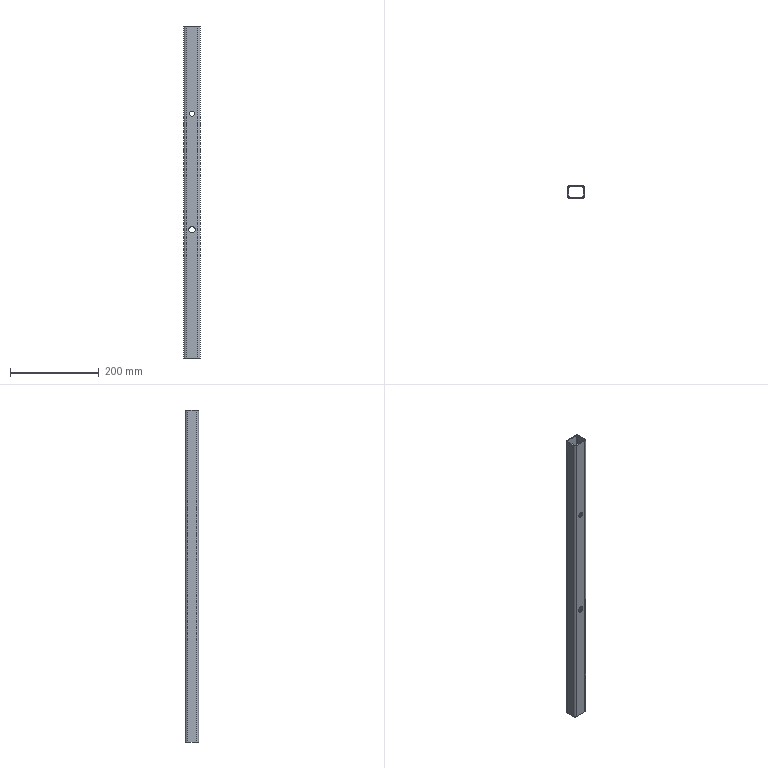Part | SolidWorks | features ICE 2, Cut 1, Extrusion 1 | 1 solid | 27 faces | box 37 x 30 x 750 mm | volume 218758 mm3 | cylinder 16 | plane 11 | commonest cylinder face diameters 5 x4 10 x4 12 x4 14 x4
STEP:
#1=CARTESIAN_POINT('',(7.,12.5,-260.));
#2=VERTEX_POINT('',#1);
#3=CARTESIAN_POINT('',(-7.,12.5,-260.));
#4=VERTEX_POINT('',#3);
#5=CARTESIAN_POINT('',(0.,12.5,-260.));
#6=DIRECTION('',(0.,1.,0.));
#7=DIRECTION('',(-1.,0.,0.));
#8=AXIS2_PLACEMENT_3D('',#5,#6,#7);
#9=CIRCLE('',#8,7.);
#10=EDGE_CURVE('',#2,#4,#9,.T.);
#11=ORIENTED_EDGE('',*,*,#10,.F.);
#12=CARTESIAN_POINT('',(7.,15.,-260.));
#13=VERTEX_POINT('',#12);
#14=CARTESIAN_POINT('',(7.,-15.,-260.));
#15=DIRECTION('',(0.,1.,0.));
#16=VECTOR('',#15,1000.);
#17=LINE('',#14,#16);
#18=EDGE_CURVE('',#2,#13,#17,.T.);
#19=ORIENTED_EDGE('',*,*,#18,.T.);
#20=CARTESIAN_POINT('',(-7.,15.,-260.));
#21=VERTEX_POINT('',#20);
#22=CARTESIAN_POINT('',(0.,15.,-260.));
#23=DIRECTION('',(0.,1.,0.));
#24=DIRECTION('',(-1.,0.,0.));
#25=AXIS2_PLACEMENT_3D('',#22,#23,#24);
#26=CIRCLE('',#25,7.);
#27=EDGE_CURVE('',#13,#21,#26,.T.);
#28=ORIENTED_EDGE('',*,*,#27,.T.);
#29=CARTESIAN_POINT('',(-7.,-15.,-260.));
#30=DIRECTION('',(0.,1.,0.));
#31=VECTOR('',#30,1000.);
#32=LINE('',#29,#31);
#33=EDGE_CURVE('',#4,#21,#32,.T.);
#34=ORIENTED_EDGE('',*,*,#33,.F.);
#35=EDGE_LOOP('',(#11,#19,#28,#34));
#36=FACE_OUTER_BOUND('',#35,.T.);
#37=CARTESIAN_POINT('',(0.,-15.,-260.));
#38=DIRECTION('',(0.,1.,0.));
#39=DIRECTION('',(-1.,0.,0.));
#40=AXIS2_PLACEMENT_3D('',#37,#38,#39);
#41=CYLINDRICAL_SURFACE('',#40,7.);
#42=ADVANCED_FACE('',(#36),#41,.F.);
#43=CARTESIAN_POINT('',(7.,-15.,-260.));
#44=VERTEX_POINT('',#43);
#45=CARTESIAN_POINT('',(-7.,-15.,-260.));
#46=VERTEX_POINT('',#45);
#47=CARTESIAN_POINT('',(0.,-15.,-260.));
#48=DIRECTION('',(0.,1.,0.));
#49=DIRECTION('',(-1.,0.,0.));
#50=AXIS2_PLACEMENT_3D('',#47,#48,#49);
#51=CIRCLE('',#50,7.);
#52=EDGE_CURVE('',#44,#46,#51,.T.);
#53=ORIENTED_EDGE('',*,*,#52,.F.);
#54=CARTESIAN_POINT('',(7.,-12.5,-260.));
#55=VERTEX_POINT('',#54);
#56=CARTESIAN_POINT('',(7.,-15.,-260.));
#57=DIRECTION('',(0.,1.,0.));
#58=VECTOR('',#57,1000.);
#59=LINE('',#56,#58);
#60=EDGE_CURVE('',#44,#55,#59,.T.);
#61=ORIENTED_EDGE('',*,*,#60,.T.);
#62=CARTESIAN_POINT('',(-7.,-12.5,-260.));
#63=VERTEX_POINT('',#62);
#64=CARTESIAN_POINT('',(0.,-12.5,-260.));
#65=DIRECTION('',(0.,-1.,0.));
#66=DIRECTION('',(1.,0.,0.));
#67=AXIS2_PLACEMENT_3D('',#64,#65,#66);
#68=CIRCLE('',#67,7.);
#69=EDGE_CURVE('',#63,#55,#68,.T.);
#70=ORIENTED_EDGE('',*,*,#69,.F.);
#71=CARTESIAN_POINT('',(-7.,-15.,-260.));
#72=DIRECTION('',(0.,1.,0.));
#73=VECTOR('',#72,1000.);
#74=LINE('',#71,#73);
#75=EDGE_CURVE('',#46,#63,#74,.T.);
#76=ORIENTED_EDGE('',*,*,#75,.F.);
#77=EDGE_LOOP('',(#53,#61,#70,#76));
#78=FACE_OUTER_BOUND('',#77,.T.);
#79=CARTESIAN_POINT('',(0.,-15.,-260.));
#80=DIRECTION('',(0.,1.,0.));
#81=DIRECTION('',(-1.,0.,0.));
#82=AXIS2_PLACEMENT_3D('',#79,#80,#81);
#83=CYLINDRICAL_SURFACE('',#82,7.);
#84=ADVANCED_FACE('',(#78),#83,.F.);
#85=CARTESIAN_POINT('',(6.,12.5,2.));
#86=VERTEX_POINT('',#85);
#87=CARTESIAN_POINT('',(-6.,12.5,2.));
#88=VERTEX_POINT('',#87);
#89=CARTESIAN_POINT('',(0.,12.5,2.));
#90=DIRECTION('',(0.,1.,0.));
#91=DIRECTION('',(-1.,0.,0.));
#92=AXIS2_PLACEMENT_3D('',#89,#90,#91);
#93=CIRCLE('',#92,6.);
#94=EDGE_CURVE('',#86,#88,#93,.T.);
#95=ORIENTED_EDGE('',*,*,#94,.F.);
#96=CARTESIAN_POINT('',(6.,15.,2.));
#97=VERTEX_POINT('',#96);
#98=CARTESIAN_POINT('',(6.,-68.,2.));
#99=DIRECTION('',(0.,1.,0.));
#100=VECTOR('',#99,1000.);
#101=LINE('',#98,#100);
#102=EDGE_CURVE('',#86,#97,#101,.T.);
#103=ORIENTED_EDGE('',*,*,#102,.T.);
#104=CARTESIAN_POINT('',(-6.,15.,2.));
#105=VERTEX_POINT('',#104);
#106=CARTESIAN_POINT('',(0.,15.,2.));
#107=DIRECTION('',(0.,1.,0.));
#108=DIRECTION('',(-1.,0.,0.));
#109=AXIS2_PLACEMENT_3D('',#106,#107,#108);
#110=CIRCLE('',#109,6.);
#111=EDGE_CURVE('',#97,#105,#110,.T.);
#112=ORIENTED_EDGE('',*,*,#111,.T.);
#113=CARTESIAN_POINT('',(-6.,-68.,2.));
#114=DIRECTION('',(0.,1.,0.));
#115=VECTOR('',#114,1000.);
#116=LINE('',#113,#115);
#117=EDGE_CURVE('',#88,#105,#116,.T.);
#118=ORIENTED_EDGE('',*,*,#117,.F.);
#119=EDGE_LOOP('',(#95,#103,#112,#118));
#120=FACE_OUTER_BOUND('',#119,.T.);
#121=CARTESIAN_POINT('',(0.,-68.,2.));
#122=DIRECTION('',(0.,1.,0.));
#123=DIRECTION('',(-1.,0.,0.));
#124=AXIS2_PLACEMENT_3D('',#121,#122,#123);
#125=CYLINDRICAL_SURFACE('',#124,6.);
#126=ADVANCED_FACE('',(#120),#125,.F.);
#127=CARTESIAN_POINT('',(-6.,-15.,2.));
#128=VERTEX_POINT('',#127);
#129=CARTESIAN_POINT('',(6.,-15.,2.));
#130=VERTEX_POINT('',#129);
#131=CARTESIAN_POINT('',(0.,-15.,2.));
#132=DIRECTION('',(0.,-1.,0.));
#133=DIRECTION('',(1.,0.,0.));
#134=AXIS2_PLACEMENT_3D('',#131,#132,#133);
#135=CIRCLE('',#134,6.);
#136=EDGE_CURVE('',#128,#130,#135,.T.);
#137=ORIENTED_EDGE('',*,*,#136,.T.);
#138=CARTESIAN_POINT('',(6.,-12.5,2.));
#139=VERTEX_POINT('',#138);
#140=CARTESIAN_POINT('',(6.,-68.,2.));
#141=DIRECTION('',(0.,1.,0.));
#142=VECTOR('',#141,1000.);
#143=LINE('',#140,#142);
#144=EDGE_CURVE('',#130,#139,#143,.T.);
#145=ORIENTED_EDGE('',*,*,#144,.T.);
#146=CARTESIAN_POINT('',(-6.,-12.5,2.));
#147=VERTEX_POINT('',#146);
#148=CARTESIAN_POINT('',(0.,-12.5,2.));
#149=DIRECTION('',(0.,-1.,0.));
#150=DIRECTION('',(1.,0.,0.));
#151=AXIS2_PLACEMENT_3D('',#148,#149,#150);
#152=CIRCLE('',#151,6.);
#153=EDGE_CURVE('',#147,#139,#152,.T.);
#154=ORIENTED_EDGE('',*,*,#153,.F.);
#155=CARTESIAN_POINT('',(-6.,-68.,2.));
#156=DIRECTION('',(0.,1.,0.));
#157=VECTOR('',#156,1000.);
#158=LINE('',#155,#157);
#159=EDGE_CURVE('',#128,#147,#158,.T.);
#160=ORIENTED_EDGE('',*,*,#159,.F.);
#161=EDGE_LOOP('',(#137,#145,#154,#160));
#162=FACE_OUTER_BOUND('',#161,.T.);
#163=CARTESIAN_POINT('',(0.,-68.,2.));
#164=DIRECTION('',(0.,1.,0.));
#165=DIRECTION('',(-1.,0.,0.));
#166=AXIS2_PLACEMENT_3D('',#163,#164,#165);
#167=CYLINDRICAL_SURFACE('',#166,6.);
#168=ADVANCED_FACE('',(#162),#167,.F.);
#169=CARTESIAN_POINT('',(-13.5,-15.,-550.));
#170=VERTEX_POINT('',#169);
#171=CARTESIAN_POINT('',(-13.5,-15.,200.));
#172=VERTEX_POINT('',#171);
#173=CARTESIAN_POINT('',(-13.5,-15.,-300.));
#174=DIRECTION('',(0.,0.,1.));
#175=VECTOR('',#174,1000.);
#176=LINE('',#173,#175);
#177=EDGE_CURVE('',#170,#172,#176,.T.);
#178=ORIENTED_EDGE('',*,*,#177,.T.);
#179=CARTESIAN_POINT('',(-18.5,-10.,200.));
#180=VERTEX_POINT('',#179);
#181=CARTESIAN_POINT('',(-13.5,-10.,200.));
#182=DIRECTION('',(0.,0.,1.));
#183=DIRECTION('',(1.,0.,0.));
#184=AXIS2_PLACEMENT_3D('',#181,#182,#183);
#185=CIRCLE('',#184,5.);
#186=EDGE_CURVE('',#180,#172,#185,.T.);
#187=ORIENTED_EDGE('',*,*,#186,.F.);
#188=CARTESIAN_POINT('',(-18.5,-10.,-550.));
#189=VERTEX_POINT('',#188);
#190=CARTESIAN_POINT('',(-18.5,-10.,-300.));
#191=DIRECTION('',(0.,0.,1.));
#192=VECTOR('',#191,1000.);
#193=LINE('',#190,#192);
#194=EDGE_CURVE('',#189,#180,#193,.T.);
#195=ORIENTED_EDGE('',*,*,#194,.F.);
#196=CARTESIAN_POINT('',(-13.5,-10.,-550.));
#197=DIRECTION('',(0.,0.,-1.));
#198=DIRECTION('',(-1.,0.,0.));
#199=AXIS2_PLACEMENT_3D('',#196,#197,#198);
#200=CIRCLE('',#199,5.);
#201=EDGE_CURVE('',#170,#189,#200,.T.);
#202=ORIENTED_EDGE('',*,*,#201,.F.);
#203=EDGE_LOOP('',(#178,#187,#195,#202));
#204=FACE_OUTER_BOUND('',#203,.T.);
#205=CARTESIAN_POINT('',(-13.5,-10.,-300.));
#206=DIRECTION('',(0.,0.,1.));
#207=DIRECTION('',(1.,0.,0.));
#208=AXIS2_PLACEMENT_3D('',#205,#206,#207);
#209=CYLINDRICAL_SURFACE('',#208,5.);
#210=ADVANCED_FACE('',(#204),#209,.T.);
#211=ORIENTED_EDGE('',*,*,#194,.T.);
#212=CARTESIAN_POINT('',(-18.5,10.,200.));
#213=VERTEX_POINT('',#212);
#214=CARTESIAN_POINT('',(-18.5,10.,200.));
#215=DIRECTION('',(0.,-1.,0.));
#216=VECTOR('',#215,1000.);
#217=LINE('',#214,#216);
#218=EDGE_CURVE('',#213,#180,#217,.T.);
#219=ORIENTED_EDGE('',*,*,#218,.F.);
#220=CARTESIAN_POINT('',(-18.5,10.,-550.));
#221=VERTEX_POINT('',#220);
#222=CARTESIAN_POINT('',(-18.5,10.,-300.));
#223=DIRECTION('',(0.,0.,1.));
#224=VECTOR('',#223,1000.);
#225=LINE('',#222,#224);
#226=EDGE_CURVE('',#221,#213,#225,.T.);
#227=ORIENTED_EDGE('',*,*,#226,.F.);
#228=CARTESIAN_POINT('',(-18.5,-10.,-550.));
#229=DIRECTION('',(0.,1.,0.));
#230=VECTOR('',#229,1000.);
#231=LINE('',#228,#230);
#232=EDGE_CURVE('',#189,#221,#231,.T.);
#233=ORIENTED_EDGE('',*,*,#232,.F.);
#234=EDGE_LOOP('',(#211,#219,#227,#233));
#235=FACE_OUTER_BOUND('',#234,.T.);
#236=CARTESIAN_POINT('',(-18.5,10.,-300.));
#237=DIRECTION('',(-1.,0.,0.));
#238=DIRECTION('',(0.,0.,1.));
#239=AXIS2_PLACEMENT_3D('',#236,#237,#238);
#240=PLANE('',#239);
#241=ADVANCED_FACE('',(#235),#240,.T.);
#242=ORIENTED_EDGE('',*,*,#226,.T.);
#243=CARTESIAN_POINT('',(-13.5,15.,200.));
#244=VERTEX_POINT('',#243);
#245=CARTESIAN_POINT('',(-13.5,10.,200.));
#246=DIRECTION('',(0.,0.,1.));
#247=DIRECTION('',(1.,0.,0.));
#248=AXIS2_PLACEMENT_3D('',#245,#246,#247);
#249=CIRCLE('',#248,5.);
#250=EDGE_CURVE('',#244,#213,#249,.T.);
#251=ORIENTED_EDGE('',*,*,#250,.F.);
#252=CARTESIAN_POINT('',(-13.5,15.,-550.));
#253=VERTEX_POINT('',#252);
#254=CARTESIAN_POINT('',(-13.5,15.,-300.));
#255=DIRECTION('',(0.,0.,1.));
#256=VECTOR('',#255,1000.);
#257=LINE('',#254,#256);
#258=EDGE_CURVE('',#253,#244,#257,.T.);
#259=ORIENTED_EDGE('',*,*,#258,.F.);
#260=CARTESIAN_POINT('',(-13.5,10.,-550.));
#261=DIRECTION('',(0.,0.,-1.));
#262=DIRECTION('',(-1.,0.,0.));
#263=AXIS2_PLACEMENT_3D('',#260,#261,#262);
#264=CIRCLE('',#263,5.);
#265=EDGE_CURVE('',#221,#253,#264,.T.);
#266=ORIENTED_EDGE('',*,*,#265,.F.);
#267=EDGE_LOOP('',(#242,#251,#259,#266));
#268=FACE_OUTER_BOUND('',#267,.T.);
#269=CARTESIAN_POINT('',(-13.5,10.,-300.));
#270=DIRECTION('',(0.,0.,1.));
#271=DIRECTION('',(1.,0.,0.));
#272=AXIS2_PLACEMENT_3D('',#269,#270,#271);
#273=CYLINDRICAL_SURFACE('',#272,5.);
#274=ADVANCED_FACE('',(#268),#273,.T.);
#275=CARTESIAN_POINT('',(0.,15.,-260.));
#276=DIRECTION('',(0.,1.,0.));
#277=DIRECTION('',(-1.,0.,0.));
#278=AXIS2_PLACEMENT_3D('',#275,#276,#277);
#279=CIRCLE('',#278,7.);
#280=EDGE_CURVE('',#21,#13,#279,.T.);
#281=ORIENTED_EDGE('',*,*,#280,.F.);
#282=ORIENTED_EDGE('',*,*,#27,.F.);
#283=EDGE_LOOP('',(#281,#282));
#284=FACE_BOUND('',#283,.T.);
#285=CARTESIAN_POINT('',(0.,15.,2.));
#286=DIRECTION('',(0.,1.,0.));
#287=DIRECTION('',(-1.,0.,0.));
#288=AXIS2_PLACEMENT_3D('',#285,#286,#287);
#289=CIRCLE('',#288,6.);
#290=EDGE_CURVE('',#105,#97,#289,.T.);
#291=ORIENTED_EDGE('',*,*,#290,.F.);
#292=ORIENTED_EDGE('',*,*,#111,.F.);
#293=EDGE_LOOP('',(#291,#292));
#294=FACE_BOUND('',#293,.T.);
#295=ORIENTED_EDGE('',*,*,#258,.T.);
#296=CARTESIAN_POINT('',(13.5,15.,200.));
#297=VERTEX_POINT('',#296);
#298=CARTESIAN_POINT('',(-13.5,15.,200.));
#299=DIRECTION('',(-1.,0.,0.));
#300=VECTOR('',#299,1000.);
#301=LINE('',#298,#300);
#302=EDGE_CURVE('',#297,#244,#301,.T.);
#303=ORIENTED_EDGE('',*,*,#302,.F.);
#304=CARTESIAN_POINT('',(13.5,15.,-550.));
#305=VERTEX_POINT('',#304);
#306=CARTESIAN_POINT('',(13.5,15.,-300.));
#307=DIRECTION('',(0.,0.,1.));
#308=VECTOR('',#307,1000.);
#309=LINE('',#306,#308);
#310=EDGE_CURVE('',#305,#297,#309,.T.);
#311=ORIENTED_EDGE('',*,*,#310,.F.);
#312=CARTESIAN_POINT('',(-13.5,15.,-550.));
#313=DIRECTION('',(1.,0.,0.));
#314=VECTOR('',#313,1000.);
#315=LINE('',#312,#314);
#316=EDGE_CURVE('',#253,#305,#315,.T.);
#317=ORIENTED_EDGE('',*,*,#316,.F.);
#318=EDGE_LOOP('',(#295,#303,#311,#317));
#319=FACE_OUTER_BOUND('',#318,.T.);
#320=CARTESIAN_POINT('',(-13.5,15.,-300.));
#321=DIRECTION('',(0.,1.,0.));
#322=DIRECTION('',(-1.,0.,0.));
#323=AXIS2_PLACEMENT_3D('',#320,#321,#322);
#324=PLANE('',#323);
#325=ADVANCED_FACE('',(#284,#294,#319),#324,.T.);
#326=ORIENTED_EDGE('',*,*,#310,.T.);
#327=CARTESIAN_POINT('',(18.5,10.,200.));
#328=VERTEX_POINT('',#327);
#329=CARTESIAN_POINT('',(13.5,10.,200.));
#330=DIRECTION('',(0.,0.,1.));
#331=DIRECTION('',(-1.,0.,0.));
#332=AXIS2_PLACEMENT_3D('',#329,#330,#331);
#333=CIRCLE('',#332,5.);
#334=EDGE_CURVE('',#328,#297,#333,.T.);
#335=ORIENTED_EDGE('',*,*,#334,.F.);
#336=CARTESIAN_POINT('',(18.5,10.,-550.));
#337=VERTEX_POINT('',#336);
#338=CARTESIAN_POINT('',(18.5,10.,-300.));
#339=DIRECTION('',(0.,0.,1.));
#340=VECTOR('',#339,1000.);
#341=LINE('',#338,#340);
#342=EDGE_CURVE('',#337,#328,#341,.T.);
#343=ORIENTED_EDGE('',*,*,#342,.F.);
#344=CARTESIAN_POINT('',(13.5,10.,-550.));
#345=DIRECTION('',(0.,0.,-1.));
#346=DIRECTION('',(-1.,0.,0.));
#347=AXIS2_PLACEMENT_3D('',#344,#345,#346);
#348=CIRCLE('',#347,5.);
#349=EDGE_CURVE('',#305,#337,#348,.T.);
#350=ORIENTED_EDGE('',*,*,#349,.F.);
#351=EDGE_LOOP('',(#326,#335,#343,#350));
#352=FACE_OUTER_BOUND('',#351,.T.);
#353=CARTESIAN_POINT('',(13.5,10.,-300.));
#354=DIRECTION('',(0.,0.,1.));
#355=DIRECTION('',(1.,0.,0.));
#356=AXIS2_PLACEMENT_3D('',#353,#354,#355);
#357=CYLINDRICAL_SURFACE('',#356,5.);
#358=ADVANCED_FACE('',(#352),#357,.T.);
#359=ORIENTED_EDGE('',*,*,#342,.T.);
#360=CARTESIAN_POINT('',(18.5,-10.,200.));
#361=VERTEX_POINT('',#360);
#362=CARTESIAN_POINT('',(18.5,10.,200.));
#363=DIRECTION('',(0.,1.,0.));
#364=VECTOR('',#363,1000.);
#365=LINE('',#362,#364);
#366=EDGE_CURVE('',#361,#328,#365,.T.);
#367=ORIENTED_EDGE('',*,*,#366,.F.);
#368=CARTESIAN_POINT('',(18.5,-10.,-550.));
#369=VERTEX_POINT('',#368);
#370=CARTESIAN_POINT('',(18.5,-10.,-300.));
#371=DIRECTION('',(0.,0.,1.));
#372=VECTOR('',#371,1000.);
#373=LINE('',#370,#372);
#374=EDGE_CURVE('',#369,#361,#373,.T.);
#375=ORIENTED_EDGE('',*,*,#374,.F.);
#376=CARTESIAN_POINT('',(18.5,10.,-550.));
#377=DIRECTION('',(0.,-1.,0.));
#378=VECTOR('',#377,1000.);
#379=LINE('',#376,#378);
#380=EDGE_CURVE('',#337,#369,#379,.T.);
#381=ORIENTED_EDGE('',*,*,#380,.F.);
#382=EDGE_LOOP('',(#359,#367,#375,#381));
#383=FACE_OUTER_BOUND('',#382,.T.);
#384=CARTESIAN_POINT('',(18.5,10.,-300.));
#385=DIRECTION('',(1.,0.,0.));
#386=DIRECTION('',(0.,0.,-1.));
#387=AXIS2_PLACEMENT_3D('',#384,#385,#386);
#388=PLANE('',#387);
#389=ADVANCED_FACE('',(#383),#388,.T.);
#390=ORIENTED_EDGE('',*,*,#374,.T.);
#391=CARTESIAN_POINT('',(13.5,-15.,200.));
#392=VERTEX_POINT('',#391);
#393=CARTESIAN_POINT('',(13.5,-10.,200.));
#394=DIRECTION('',(0.,0.,1.));
#395=DIRECTION('',(1.,0.,0.));
#396=AXIS2_PLACEMENT_3D('',#393,#394,#395);
#397=CIRCLE('',#396,5.);
#398=EDGE_CURVE('',#392,#361,#397,.T.);
#399=ORIENTED_EDGE('',*,*,#398,.F.);
#400=CARTESIAN_POINT('',(13.5,-15.,-550.));
#401=VERTEX_POINT('',#400);
#402=CARTESIAN_POINT('',(13.5,-15.,-300.));
#403=DIRECTION('',(0.,0.,1.));
#404=VECTOR('',#403,1000.);
#405=LINE('',#402,#404);
#406=EDGE_CURVE('',#401,#392,#405,.T.);
#407=ORIENTED_EDGE('',*,*,#406,.F.);
#408=CARTESIAN_POINT('',(13.5,-10.,-550.));
#409=DIRECTION('',(0.,0.,-1.));
#410=DIRECTION('',(-1.,0.,0.));
#411=AXIS2_PLACEMENT_3D('',#408,#409,#410);
#412=CIRCLE('',#411,5.);
#413=EDGE_CURVE('',#369,#401,#412,.T.);
#414=ORIENTED_EDGE('',*,*,#413,.F.);
#415=EDGE_LOOP('',(#390,#399,#407,#414));
#416=FACE_OUTER_BOUND('',#415,.T.);
#417=CARTESIAN_POINT('',(13.5,-10.,-300.));
#418=DIRECTION('',(0.,0.,1.));
#419=DIRECTION('',(1.,0.,0.));
#420=AXIS2_PLACEMENT_3D('',#417,#418,#419);
#421=CYLINDRICAL_SURFACE('',#420,5.);
#422=ADVANCED_FACE('',(#416),#421,.T.);
#423=CARTESIAN_POINT('',(0.,-15.,-260.));
#424=DIRECTION('',(0.,1.,0.));
#425=DIRECTION('',(-1.,0.,0.));
#426=AXIS2_PLACEMENT_3D('',#423,#424,#425);
#427=CIRCLE('',#426,7.);
#428=EDGE_CURVE('',#46,#44,#427,.T.);
#429=ORIENTED_EDGE('',*,*,#428,.T.);
#430=ORIENTED_EDGE('',*,*,#52,.T.);
#431=EDGE_LOOP('',(#429,#430));
#432=FACE_BOUND('',#431,.T.);
#433=ORIENTED_EDGE('',*,*,#136,.F.);
#434=CARTESIAN_POINT('',(0.,-15.,2.));
#435=DIRECTION('',(0.,-1.,0.));
#436=DIRECTION('',(1.,0.,0.));
#437=AXIS2_PLACEMENT_3D('',#434,#435,#436);
#438=CIRCLE('',#437,6.);
#439=EDGE_CURVE('',#130,#128,#438,.T.);
#440=ORIENTED_EDGE('',*,*,#439,.F.);
#441=EDGE_LOOP('',(#433,#440));
#442=FACE_BOUND('',#441,.T.);
#443=ORIENTED_EDGE('',*,*,#406,.T.);
#444=CARTESIAN_POINT('',(-13.5,-15.,200.));
#445=DIRECTION('',(1.,0.,0.));
#446=VECTOR('',#445,1000.);
#447=LINE('',#444,#446);
#448=EDGE_CURVE('',#172,#392,#447,.T.);
#449=ORIENTED_EDGE('',*,*,#448,.F.);
#450=ORIENTED_EDGE('',*,*,#177,.F.);
#451=CARTESIAN_POINT('',(13.5,-15.,-550.));
#452=DIRECTION('',(-1.,0.,0.));
#453=VECTOR('',#452,1000.);
#454=LINE('',#451,#453);
#455=EDGE_CURVE('',#401,#170,#454,.T.);
#456=ORIENTED_EDGE('',*,*,#455,.F.);
#457=EDGE_LOOP('',(#443,#449,#450,#456));
#458=FACE_OUTER_BOUND('',#457,.T.);
#459=CARTESIAN_POINT('',(-13.5,-15.,-300.));
#460=DIRECTION('',(0.,-1.,0.));
#461=DIRECTION('',(1.,0.,0.));
#462=AXIS2_PLACEMENT_3D('',#459,#460,#461);
#463=PLANE('',#462);
#464=ADVANCED_FACE('',(#432,#442,#458),#463,.T.);
#465=CARTESIAN_POINT('',(13.5,-12.5,-300.));
#466=VERTEX_POINT('',#465);
#467=CARTESIAN_POINT('',(16.,-10.,-300.));
#468=VERTEX_POINT('',#467);
#469=CARTESIAN_POINT('',(13.5,-10.,-300.));
#470=DIRECTION('',(0.,0.,1.));
#471=DIRECTION('',(-1.,0.,0.));
#472=AXIS2_PLACEMENT_3D('',#469,#470,#471);
#473=CIRCLE('',#472,2.5);
#474=EDGE_CURVE('',#466,#468,#473,.T.);
#475=ORIENTED_EDGE('',*,*,#474,.T.);
#476=CARTESIAN_POINT('',(16.,-12.5,-300.));
#477=VERTEX_POINT('',#476);
#478=CARTESIAN_POINT('',(16.,-12.5,-300.));
#479=DIRECTION('',(0.,-1.,0.));
#480=VECTOR('',#479,1000.);
#481=LINE('',#478,#480);
#482=EDGE_CURVE('',#468,#477,#481,.T.);
#483=ORIENTED_EDGE('',*,*,#482,.T.);
#484=CARTESIAN_POINT('',(16.,-12.5,-300.));
#485=DIRECTION('',(-1.,0.,0.));
#486=VECTOR('',#485,1000.);
#487=LINE('',#484,#486);
#488=EDGE_CURVE('',#477,#466,#487,.T.);
#489=ORIENTED_EDGE('',*,*,#488,.T.);
#490=EDGE_LOOP('',(#475,#483,#489));
#491=FACE_OUTER_BOUND('',#490,.T.);
#492=CARTESIAN_POINT('',(-13.5,-10.,-300.));
#493=DIRECTION('',(0.,0.,1.));
#494=DIRECTION('',(1.,0.,0.));
#495=AXIS2_PLACEMENT_3D('',#492,#493,#494);
#496=PLANE('',#495);
#497=ADVANCED_FACE('',(#491),#496,.F.);
#498=CARTESIAN_POINT('',(-16.,-10.,-550.));
#499=VERTEX_POINT('',#498);
#500=CARTESIAN_POINT('',(-16.,-10.,200.));
#501=VERTEX_POINT('',#500);
#502=CARTESIAN_POINT('',(-16.,-10.,-300.));
#503=DIRECTION('',(0.,0.,1.));
#504=VECTOR('',#503,1000.);
#505=LINE('',#502,#504);
#506=EDGE_CURVE('',#499,#501,#505,.T.);
#507=ORIENTED_EDGE('',*,*,#506,.T.);
#508=CARTESIAN_POINT('',(-13.5,-12.5,200.));
#509=VERTEX_POINT('',#508);
#510=CARTESIAN_POINT('',(-13.5,-10.,200.));
#511=DIRECTION('',(0.,0.,1.));
#512=DIRECTION('',(-1.,0.,0.));
#513=AXIS2_PLACEMENT_3D('',#510,#511,#512);
#514=CIRCLE('',#513,2.5);
#515=EDGE_CURVE('',#501,#509,#514,.T.);
#516=ORIENTED_EDGE('',*,*,#515,.T.);
#517=CARTESIAN_POINT('',(-13.5,-12.5,-550.));
#518=VERTEX_POINT('',#517);
#519=CARTESIAN_POINT('',(-13.5,-12.5,-300.));
#520=DIRECTION('',(0.,0.,1.));
#521=VECTOR('',#520,1000.);
#522=LINE('',#519,#521);
#523=EDGE_CURVE('',#518,#509,#522,.T.);
#524=ORIENTED_EDGE('',*,*,#523,.F.);
#525=CARTESIAN_POINT('',(-13.5,-10.,-550.));
#526=DIRECTION('',(0.,0.,-1.));
#527=DIRECTION('',(-1.,0.,0.));
#528=AXIS2_PLACEMENT_3D('',#525,#526,#527);
#529=CIRCLE('',#528,2.5);
#530=EDGE_CURVE('',#518,#499,#529,.T.);
#531=ORIENTED_EDGE('',*,*,#530,.T.);
#532=EDGE_LOOP('',(#507,#516,#524,#531));
#533=FACE_OUTER_BOUND('',#532,.T.);
#534=CARTESIAN_POINT('',(-13.5,-10.,-300.));
#535=DIRECTION('',(0.,0.,1.));
#536=DIRECTION('',(1.,0.,0.));
#537=AXIS2_PLACEMENT_3D('',#534,#535,#536);
#538=CYLINDRICAL_SURFACE('',#537,2.5);
#539=ADVANCED_FACE('',(#533),#538,.F.);
#540=CARTESIAN_POINT('',(-16.,10.,-550.));
#541=VERTEX_POINT('',#540);
#542=CARTESIAN_POINT('',(-16.,10.,200.));
#543=VERTEX_POINT('',#542);
#544=CARTESIAN_POINT('',(-16.,10.,-300.));
#545=DIRECTION('',(0.,0.,1.));
#546=VECTOR('',#545,1000.);
#547=LINE('',#544,#546);
#548=EDGE_CURVE('',#541,#543,#547,.T.);
#549=ORIENTED_EDGE('',*,*,#548,.T.);
#550=CARTESIAN_POINT('',(-16.,10.,200.));
#551=DIRECTION('',(0.,-1.,0.));
#552=VECTOR('',#551,1000.);
#553=LINE('',#550,#552);
#554=EDGE_CURVE('',#543,#501,#553,.T.);
#555=ORIENTED_EDGE('',*,*,#554,.T.);
#556=ORIENTED_EDGE('',*,*,#506,.F.);
#557=CARTESIAN_POINT('',(-16.,-10.,-550.));
#558=DIRECTION('',(0.,1.,0.));
#559=VECTOR('',#558,1000.);
#560=LINE('',#557,#559);
#561=EDGE_CURVE('',#499,#541,#560,.T.);
#562=ORIENTED_EDGE('',*,*,#561,.T.);
#563=EDGE_LOOP('',(#549,#555,#556,#562));
#564=FACE_OUTER_BOUND('',#563,.T.);
#565=CARTESIAN_POINT('',(-16.,10.,-300.));
#566=DIRECTION('',(-1.,0.,0.));
#567=DIRECTION('',(0.,0.,1.));
#568=AXIS2_PLACEMENT_3D('',#565,#566,#567);
#569=PLANE('',#568);
#570=ADVANCED_FACE('',(#564),#569,.F.);
#571=CARTESIAN_POINT('',(-13.5,12.5,-550.));
#572=VERTEX_POINT('',#571);
#573=CARTESIAN_POINT('',(-13.5,12.5,200.));
#574=VERTEX_POINT('',#573);
#575=CARTESIAN_POINT('',(-13.5,12.5,-300.));
#576=DIRECTION('',(0.,0.,1.));
#577=VECTOR('',#576,1000.);
#578=LINE('',#575,#577);
#579=EDGE_CURVE('',#572,#574,#578,.T.);
#580=ORIENTED_EDGE('',*,*,#579,.T.);
#581=CARTESIAN_POINT('',(-13.5,10.,200.));
#582=DIRECTION('',(0.,0.,1.));
#583=DIRECTION('',(1.,0.,0.));
#584=AXIS2_PLACEMENT_3D('',#581,#582,#583);
#585=CIRCLE('',#584,2.5);
#586=EDGE_CURVE('',#574,#543,#585,.T.);
#587=ORIENTED_EDGE('',*,*,#586,.T.);
#588=ORIENTED_EDGE('',*,*,#548,.F.);
#589=CARTESIAN_POINT('',(-13.5,10.,-550.));
#590=DIRECTION('',(0.,0.,-1.));
#591=DIRECTION('',(-1.,0.,0.));
#592=AXIS2_PLACEMENT_3D('',#589,#590,#591);
#593=CIRCLE('',#592,2.5);
#594=EDGE_CURVE('',#541,#572,#593,.T.);
#595=ORIENTED_EDGE('',*,*,#594,.T.);
#596=EDGE_LOOP('',(#580,#587,#588,#595));
#597=FACE_OUTER_BOUND('',#596,.T.);
#598=CARTESIAN_POINT('',(-13.5,10.,-300.));
#599=DIRECTION('',(0.,0.,1.));
#600=DIRECTION('',(1.,0.,0.));
#601=AXIS2_PLACEMENT_3D('',#598,#599,#600);
#602=CYLINDRICAL_SURFACE('',#601,2.5);
#603=ADVANCED_FACE('',(#597),#602,.F.);
#604=CARTESIAN_POINT('',(0.,12.5,-260.));
#605=DIRECTION('',(0.,1.,0.));
#606=DIRECTION('',(-1.,0.,0.));
#607=AXIS2_PLACEMENT_3D('',#604,#605,#606);
#608=CIRCLE('',#607,7.);
#609=EDGE_CURVE('',#4,#2,#608,.T.);
#610=ORIENTED_EDGE('',*,*,#609,.T.);
#611=ORIENTED_EDGE('',*,*,#10,.T.);
#612=EDGE_LOOP('',(#610,#611));
#613=FACE_BOUND('',#612,.T.);
#614=CARTESIAN_POINT('',(0.,12.5,2.));
#615=DIRECTION('',(0.,1.,0.));
#616=DIRECTION('',(-1.,0.,0.));
#617=AXIS2_PLACEMENT_3D('',#614,#615,#616);
#618=CIRCLE('',#617,6.);
#619=EDGE_CURVE('',#88,#86,#618,.T.);
#620=ORIENTED_EDGE('',*,*,#619,.T.);
#621=ORIENTED_EDGE('',*,*,#94,.T.);
#622=EDGE_LOOP('',(#620,#621));
#623=FACE_BOUND('',#622,.T.);
#624=CARTESIAN_POINT('',(13.5,12.5,-550.));
#625=VERTEX_POINT('',#624);
#626=CARTESIAN_POINT('',(13.5,12.5,200.));
#627=VERTEX_POINT('',#626);
#628=CARTESIAN_POINT('',(13.5,12.5,-300.));
#629=DIRECTION('',(0.,0.,1.));
#630=VECTOR('',#629,1000.);
#631=LINE('',#628,#630);
#632=EDGE_CURVE('',#625,#627,#631,.T.);
#633=ORIENTED_EDGE('',*,*,#632,.T.);
#634=CARTESIAN_POINT('',(-13.5,12.5,200.));
#635=DIRECTION('',(-1.,0.,0.));
#636=VECTOR('',#635,1000.);
#637=LINE('',#634,#636);
#638=EDGE_CURVE('',#627,#574,#637,.T.);
#639=ORIENTED_EDGE('',*,*,#638,.T.);
#640=ORIENTED_EDGE('',*,*,#579,.F.);
#641=CARTESIAN_POINT('',(13.5,12.5,-550.));
#642=DIRECTION('',(1.,0.,0.));
#643=VECTOR('',#642,1000.);
#644=LINE('',#641,#643);
#645=EDGE_CURVE('',#572,#625,#644,.T.);
#646=ORIENTED_EDGE('',*,*,#645,.T.);
#647=EDGE_LOOP('',(#633,#639,#640,#646));
#648=FACE_OUTER_BOUND('',#647,.T.);
#649=CARTESIAN_POINT('',(-13.5,12.5,-300.));
#650=DIRECTION('',(0.,1.,0.));
#651=DIRECTION('',(-1.,0.,0.));
#652=AXIS2_PLACEMENT_3D('',#649,#650,#651);
#653=PLANE('',#652);
#654=ADVANCED_FACE('',(#613,#623,#648),#653,.F.);
#655=CARTESIAN_POINT('',(16.,10.,-550.));
#656=VERTEX_POINT('',#655);
#657=CARTESIAN_POINT('',(16.,10.,200.));
#658=VERTEX_POINT('',#657);
#659=CARTESIAN_POINT('',(16.,10.,-300.));
#660=DIRECTION('',(0.,0.,1.));
#661=VECTOR('',#660,1000.);
#662=LINE('',#659,#661);
#663=EDGE_CURVE('',#656,#658,#662,.T.);
#664=ORIENTED_EDGE('',*,*,#663,.T.);
#665=CARTESIAN_POINT('',(13.5,10.,200.));
#666=DIRECTION('',(0.,0.,1.));
#667=DIRECTION('',(-1.,0.,0.));
#668=AXIS2_PLACEMENT_3D('',#665,#666,#667);
#669=CIRCLE('',#668,2.5);
#670=EDGE_CURVE('',#658,#627,#669,.T.);
#671=ORIENTED_EDGE('',*,*,#670,.T.);
#672=ORIENTED_EDGE('',*,*,#632,.F.);
#673=CARTESIAN_POINT('',(13.5,10.,-550.));
#674=DIRECTION('',(0.,0.,-1.));
#675=DIRECTION('',(1.,0.,0.));
#676=AXIS2_PLACEMENT_3D('',#673,#674,#675);
#677=CIRCLE('',#676,2.5);
#678=EDGE_CURVE('',#625,#656,#677,.T.);
#679=ORIENTED_EDGE('',*,*,#678,.T.);
#680=EDGE_LOOP('',(#664,#671,#672,#679));
#681=FACE_OUTER_BOUND('',#680,.T.);
#682=CARTESIAN_POINT('',(13.5,10.,-300.));
#683=DIRECTION('',(0.,0.,1.));
#684=DIRECTION('',(1.,0.,0.));
#685=AXIS2_PLACEMENT_3D('',#682,#683,#684);
#686=CYLINDRICAL_SURFACE('',#685,2.5);
#687=ADVANCED_FACE('',(#681),#686,.F.);
#688=CARTESIAN_POINT('',(16.,-10.,200.));
#689=VERTEX_POINT('',#688);
#690=CARTESIAN_POINT('',(16.,-10.,-300.));
#691=DIRECTION('',(0.,0.,1.));
#692=VECTOR('',#691,1000.);
#693=LINE('',#690,#692);
#694=EDGE_CURVE('',#468,#689,#693,.T.);
#695=ORIENTED_EDGE('',*,*,#694,.T.);
#696=CARTESIAN_POINT('',(16.,10.,200.));
#697=DIRECTION('',(0.,1.,0.));
#698=VECTOR('',#697,1000.);
#699=LINE('',#696,#698);
#700=EDGE_CURVE('',#689,#658,#699,.T.);
#701=ORIENTED_EDGE('',*,*,#700,.T.);
#702=ORIENTED_EDGE('',*,*,#663,.F.);
#703=CARTESIAN_POINT('',(16.,-12.5,-550.));
#704=VERTEX_POINT('',#703);
#705=CARTESIAN_POINT('',(16.,-12.5,-550.));
#706=DIRECTION('',(0.,-1.,0.));
#707=VECTOR('',#706,1000.);
#708=LINE('',#705,#707);
#709=EDGE_CURVE('',#656,#704,#708,.T.);
#710=ORIENTED_EDGE('',*,*,#709,.T.);
#711=CARTESIAN_POINT('',(16.,-12.5,-550.));
#712=DIRECTION('',(0.,0.,1.));
#713=VECTOR('',#712,1000.);
#714=LINE('',#711,#713);
#715=EDGE_CURVE('',#704,#477,#714,.T.);
#716=ORIENTED_EDGE('',*,*,#715,.T.);
#717=ORIENTED_EDGE('',*,*,#482,.F.);
#718=EDGE_LOOP('',(#695,#701,#702,#710,#716,#717));
#719=FACE_OUTER_BOUND('',#718,.T.);
#720=CARTESIAN_POINT('',(16.,10.,-300.));
#721=DIRECTION('',(1.,0.,0.));
#722=DIRECTION('',(0.,0.,-1.));
#723=AXIS2_PLACEMENT_3D('',#720,#721,#722);
#724=PLANE('',#723);
#725=ADVANCED_FACE('',(#719),#724,.F.);
#726=CARTESIAN_POINT('',(13.5,-12.5,200.));
#727=VERTEX_POINT('',#726);
#728=CARTESIAN_POINT('',(13.5,-12.5,-300.));
#729=DIRECTION('',(0.,0.,1.));
#730=VECTOR('',#729,1000.);
#731=LINE('',#728,#730);
#732=EDGE_CURVE('',#466,#727,#731,.T.);
#733=ORIENTED_EDGE('',*,*,#732,.T.);
#734=CARTESIAN_POINT('',(13.5,-10.,200.));
#735=DIRECTION('',(0.,0.,1.));
#736=DIRECTION('',(-1.,0.,0.));
#737=AXIS2_PLACEMENT_3D('',#734,#735,#736);
#738=CIRCLE('',#737,2.5);
#739=EDGE_CURVE('',#727,#689,#738,.T.);
#740=ORIENTED_EDGE('',*,*,#739,.T.);
#741=ORIENTED_EDGE('',*,*,#694,.F.);
#742=ORIENTED_EDGE('',*,*,#474,.F.);
#743=EDGE_LOOP('',(#733,#740,#741,#742));
#744=FACE_OUTER_BOUND('',#743,.T.);
#745=CARTESIAN_POINT('',(13.5,-10.,-300.));
#746=DIRECTION('',(0.,0.,1.));
#747=DIRECTION('',(1.,0.,0.));
#748=AXIS2_PLACEMENT_3D('',#745,#746,#747);
#749=CYLINDRICAL_SURFACE('',#748,2.5);
#750=ADVANCED_FACE('',(#744),#749,.F.);
#751=ORIENTED_EDGE('',*,*,#69,.T.);
#752=CARTESIAN_POINT('',(0.,-12.5,-260.));
#753=DIRECTION('',(0.,-1.,0.));
#754=DIRECTION('',(1.,0.,0.));
#755=AXIS2_PLACEMENT_3D('',#752,#753,#754);
#756=CIRCLE('',#755,7.);
#757=EDGE_CURVE('',#55,#63,#756,.T.);
#758=ORIENTED_EDGE('',*,*,#757,.T.);
#759=EDGE_LOOP('',(#751,#758));
#760=FACE_BOUND('',#759,.T.);
#761=ORIENTED_EDGE('',*,*,#153,.T.);
#762=CARTESIAN_POINT('',(0.,-12.5,2.));
#763=DIRECTION('',(0.,-1.,0.));
#764=DIRECTION('',(1.,0.,0.));
#765=AXIS2_PLACEMENT_3D('',#762,#763,#764);
#766=CIRCLE('',#765,6.);
#767=EDGE_CURVE('',#139,#147,#766,.T.);
#768=ORIENTED_EDGE('',*,*,#767,.T.);
#769=EDGE_LOOP('',(#761,#768));
#770=FACE_BOUND('',#769,.T.);
#771=ORIENTED_EDGE('',*,*,#523,.T.);
#772=CARTESIAN_POINT('',(-13.5,-12.5,200.));
#773=DIRECTION('',(1.,0.,0.));
#774=VECTOR('',#773,1000.);
#775=LINE('',#772,#774);
#776=EDGE_CURVE('',#509,#727,#775,.T.);
#777=ORIENTED_EDGE('',*,*,#776,.T.);
#778=ORIENTED_EDGE('',*,*,#732,.F.);
#779=ORIENTED_EDGE('',*,*,#488,.F.);
#780=ORIENTED_EDGE('',*,*,#715,.F.);
#781=CARTESIAN_POINT('',(16.,-12.5,-550.));
#782=DIRECTION('',(-1.,0.,0.));
#783=VECTOR('',#782,1000.);
#784=LINE('',#781,#783);
#785=EDGE_CURVE('',#704,#518,#784,.T.);
#786=ORIENTED_EDGE('',*,*,#785,.T.);
#787=EDGE_LOOP('',(#771,#777,#778,#779,#780,#786));
#788=FACE_OUTER_BOUND('',#787,.T.);
#789=CARTESIAN_POINT('',(-13.5,-12.5,-300.));
#790=DIRECTION('',(0.,-1.,0.));
#791=DIRECTION('',(1.,0.,0.));
#792=AXIS2_PLACEMENT_3D('',#789,#790,#791);
#793=PLANE('',#792);
#794=ADVANCED_FACE('',(#760,#770,#788),#793,.F.);
#795=ORIENTED_EDGE('',*,*,#186,.T.);
#796=ORIENTED_EDGE('',*,*,#448,.T.);
#797=ORIENTED_EDGE('',*,*,#398,.T.);
#798=ORIENTED_EDGE('',*,*,#366,.T.);
#799=ORIENTED_EDGE('',*,*,#334,.T.);
#800=ORIENTED_EDGE('',*,*,#302,.T.);
#801=ORIENTED_EDGE('',*,*,#250,.T.);
#802=ORIENTED_EDGE('',*,*,#218,.T.);
#803=EDGE_LOOP('',(#795,#796,#797,#798,#799,#800,#801,#802));
#804=FACE_OUTER_BOUND('',#803,.T.);
#805=ORIENTED_EDGE('',*,*,#776,.F.);
#806=ORIENTED_EDGE('',*,*,#515,.F.);
#807=ORIENTED_EDGE('',*,*,#554,.F.);
#808=ORIENTED_EDGE('',*,*,#586,.F.);
#809=ORIENTED_EDGE('',*,*,#638,.F.);
#810=ORIENTED_EDGE('',*,*,#670,.F.);
#811=ORIENTED_EDGE('',*,*,#700,.F.);
#812=ORIENTED_EDGE('',*,*,#739,.F.);
#813=EDGE_LOOP('',(#805,#806,#807,#808,#809,#810,#811,#812));
#814=FACE_BOUND('',#813,.T.);
#815=CARTESIAN_POINT('',(-13.5,-10.,200.));
#816=DIRECTION('',(0.,0.,1.));
#817=DIRECTION('',(1.,0.,0.));
#818=AXIS2_PLACEMENT_3D('',#815,#816,#817);
#819=PLANE('',#818);
#820=ADVANCED_FACE('',(#804,#814),#819,.T.);
#821=ORIENTED_EDGE('',*,*,#144,.F.);
#822=ORIENTED_EDGE('',*,*,#439,.T.);
#823=ORIENTED_EDGE('',*,*,#159,.T.);
#824=ORIENTED_EDGE('',*,*,#767,.F.);
#825=EDGE_LOOP('',(#821,#822,#823,#824));
#826=FACE_OUTER_BOUND('',#825,.T.);
#827=CARTESIAN_POINT('',(0.,-68.,2.));
#828=DIRECTION('',(0.,1.,0.));
#829=DIRECTION('',(-1.,0.,0.));
#830=AXIS2_PLACEMENT_3D('',#827,#828,#829);
#831=CYLINDRICAL_SURFACE('',#830,6.);
#832=ADVANCED_FACE('',(#826),#831,.F.);
#833=ORIENTED_EDGE('',*,*,#102,.F.);
#834=ORIENTED_EDGE('',*,*,#619,.F.);
#835=ORIENTED_EDGE('',*,*,#117,.T.);
#836=ORIENTED_EDGE('',*,*,#290,.T.);
#837=EDGE_LOOP('',(#833,#834,#835,#836));
#838=FACE_OUTER_BOUND('',#837,.T.);
#839=CARTESIAN_POINT('',(0.,-68.,2.));
#840=DIRECTION('',(0.,1.,0.));
#841=DIRECTION('',(-1.,0.,0.));
#842=AXIS2_PLACEMENT_3D('',#839,#840,#841);
#843=CYLINDRICAL_SURFACE('',#842,6.);
#844=ADVANCED_FACE('',(#838),#843,.F.);
#845=ORIENTED_EDGE('',*,*,#60,.F.);
#846=ORIENTED_EDGE('',*,*,#428,.F.);
#847=ORIENTED_EDGE('',*,*,#75,.T.);
#848=ORIENTED_EDGE('',*,*,#757,.F.);
#849=EDGE_LOOP('',(#845,#846,#847,#848));
#850=FACE_OUTER_BOUND('',#849,.T.);
#851=CARTESIAN_POINT('',(0.,-15.,-260.));
#852=DIRECTION('',(0.,1.,0.));
#853=DIRECTION('',(-1.,0.,0.));
#854=AXIS2_PLACEMENT_3D('',#851,#852,#853);
#855=CYLINDRICAL_SURFACE('',#854,7.);
#856=ADVANCED_FACE('',(#850),#855,.F.);
#857=ORIENTED_EDGE('',*,*,#18,.F.);
#858=ORIENTED_EDGE('',*,*,#609,.F.);
#859=ORIENTED_EDGE('',*,*,#33,.T.);
#860=ORIENTED_EDGE('',*,*,#280,.T.);
#861=EDGE_LOOP('',(#857,#858,#859,#860));
#862=FACE_OUTER_BOUND('',#861,.T.);
#863=CARTESIAN_POINT('',(0.,-15.,-260.));
#864=DIRECTION('',(0.,1.,0.));
#865=DIRECTION('',(-1.,0.,0.));
#866=AXIS2_PLACEMENT_3D('',#863,#864,#865);
#867=CYLINDRICAL_SURFACE('',#866,7.);
#868=ADVANCED_FACE('',(#862),#867,.F.);
#869=ORIENTED_EDGE('',*,*,#201,.T.);
#870=ORIENTED_EDGE('',*,*,#232,.T.);
#871=ORIENTED_EDGE('',*,*,#265,.T.);
#872=ORIENTED_EDGE('',*,*,#316,.T.);
#873=ORIENTED_EDGE('',*,*,#349,.T.);
#874=ORIENTED_EDGE('',*,*,#380,.T.);
#875=ORIENTED_EDGE('',*,*,#413,.T.);
#876=ORIENTED_EDGE('',*,*,#455,.T.);
#877=EDGE_LOOP('',(#869,#870,#871,#872,#873,#874,#875,#876));
#878=FACE_OUTER_BOUND('',#877,.T.);
#879=ORIENTED_EDGE('',*,*,#785,.F.);
#880=ORIENTED_EDGE('',*,*,#709,.F.);
#881=ORIENTED_EDGE('',*,*,#678,.F.);
#882=ORIENTED_EDGE('',*,*,#645,.F.);
#883=ORIENTED_EDGE('',*,*,#594,.F.);
#884=ORIENTED_EDGE('',*,*,#561,.F.);
#885=ORIENTED_EDGE('',*,*,#530,.F.);
#886=EDGE_LOOP('',(#879,#880,#881,#882,#883,#884,#885));
#887=FACE_BOUND('',#886,.T.);
#888=CARTESIAN_POINT('',(-13.5,-10.,-550.));
#889=DIRECTION('',(0.,0.,-1.));
#890=DIRECTION('',(-1.,0.,0.));
#891=AXIS2_PLACEMENT_3D('',#888,#889,#890);
#892=PLANE('',#891);
#893=ADVANCED_FACE('',(#878,#887),#892,.T.);
#894=CLOSED_SHELL('',(#42,#84,#126,#168,#210,#241,#274,#325,#358,#389,#422,#464,#497,#539,#570,#603,#654,#687,#725,#750,#794,#820,#832,#844,#856,#868,#893));
#895=MANIFOLD_SOLID_BREP('',#894);
#896=CARTESIAN_POINT('',(0.,0.,0.));
#897=DIRECTION('',(0.,0.,1.));
#898=DIRECTION('',(1.,0.,0.));
#899=AXIS2_PLACEMENT_3D('',#896,#897,#898);
#900=(LENGTH_UNIT()NAMED_UNIT(*)SI_UNIT(.MILLI.,.METRE.));
#901=UNCERTAINTY_MEASURE_WITH_UNIT(LENGTH_MEASURE(0.00001),#900,'','');
#902=(NAMED_UNIT(*)PLANE_ANGLE_UNIT()SI_UNIT($,.RADIAN.));
#903=(NAMED_UNIT(*)SI_UNIT($,.STERADIAN.)SOLID_ANGLE_UNIT());
#904=(GEOMETRIC_REPRESENTATION_CONTEXT(3)GLOBAL_UNCERTAINTY_ASSIGNED_CONTEXT((#901))GLOBAL_UNIT_ASSIGNED_CONTEXT((#900,#902,#903))REPRESENTATION_CONTEXT('',''));
#905=ADVANCED_BREP_SHAPE_REPRESENTATION('',(#895,#899),#904);